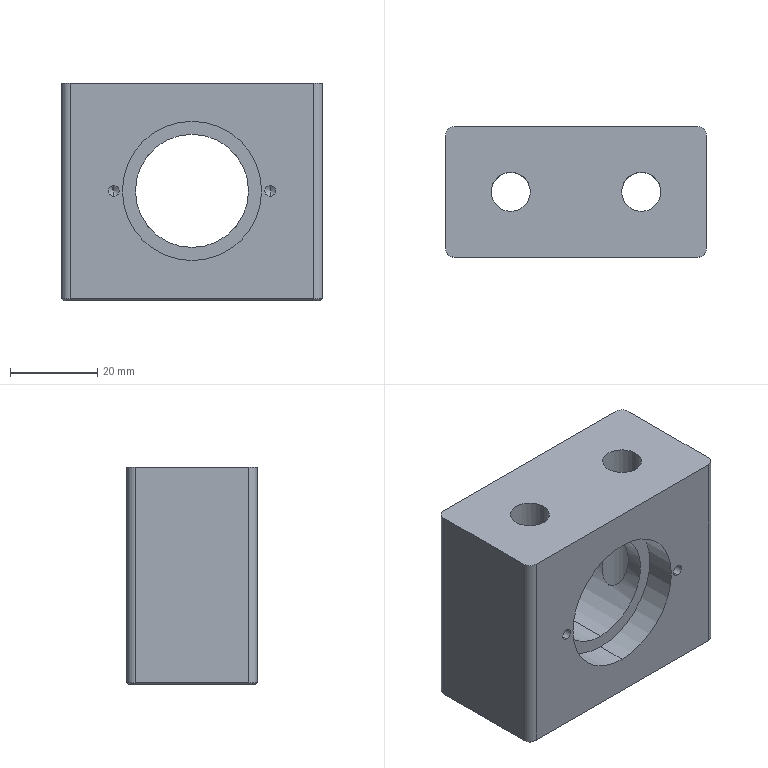Part | SolidWorks | features BaseBody 1 | 1 solid | 52 faces | box 60 x 30 x 50 mm | volume 61774 mm3 | cylinder 26 | plane 14 | cone 12 | commonest cylinder face diameters 2.5 x8 4 x4 9 x4 15 x4 32 x4 26 x2